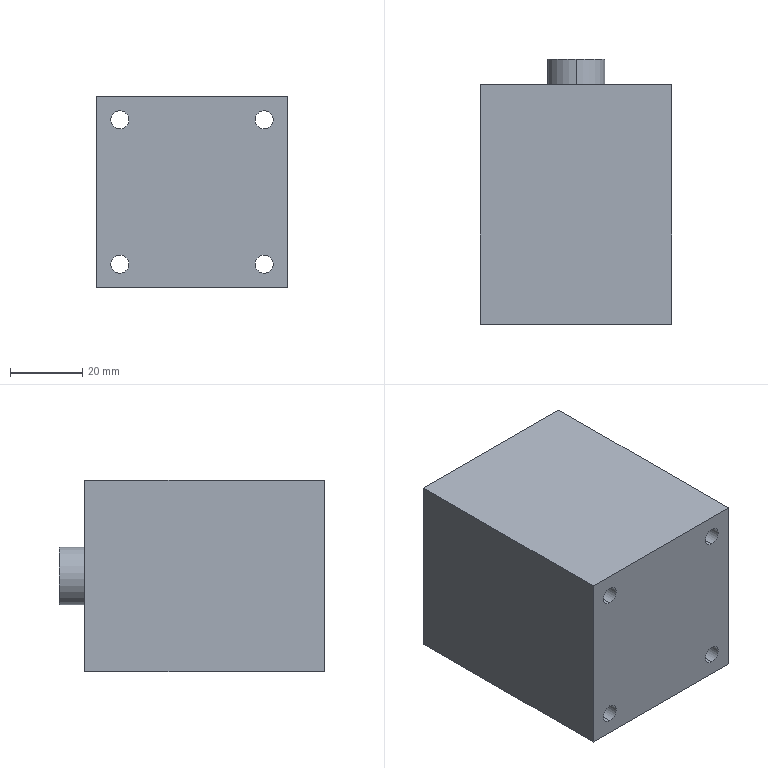Part | STEP file | 1 solid | 21 faces | box 53 x 73.5 x 53 mm | volume 182241 mm3 | cylinder 12 | plane 7 | cone 2 | commonest cylinder face diameters 5 x8 6.8 x2 16 x2
STEP:
#1=CARTESIAN_POINT('',(0.,0.,0.));
#2=DIRECTION('',(0.,0.,1.));
#3=DIRECTION('',(1.,0.,0.));
#4=AXIS2_PLACEMENT_3D('',#1,#2,#3);
#5=CARTESIAN_POINT('',(-20.,0.,-17.5));
#6=VERTEX_POINT('',#5);
#7=CARTESIAN_POINT('',(-20.,66.5,-17.5));
#8=VERTEX_POINT('',#7);
#9=CARTESIAN_POINT('',(-20.,66.5,-17.5));
#10=DIRECTION('',(0.,1.,0.));
#11=VECTOR('',#10,1.);
#12=LINE('',#9,#11);
#13=CARTESIAN_POINT('',(-20.,66.5,-20.));
#14=DIRECTION('',(0.,1.,0.));
#15=DIRECTION('',(0.,0.,1.));
#16=AXIS2_PLACEMENT_3D('',#13,#14,#15);
#17=CYLINDRICAL_SURFACE('',#16,2.5);
#18=CARTESIAN_POINT('',(6.283,0.));
#19=DIRECTION('',(0.,1.));
#20=VECTOR('',#19,1.);
#21=LINE('',#18,#20);
#22=(GEOMETRIC_REPRESENTATION_CONTEXT(2)PARAMETRIC_REPRESENTATION_CONTEXT()REPRESENTATION_CONTEXT('',''));
#23=DEFINITIONAL_REPRESENTATION('',(#21),#22);
#24=PCURVE('',#17,#23);
#25=CARTESIAN_POINT('',(-20.,66.5,-20.));
#26=DIRECTION('',(0.,1.,0.));
#27=DIRECTION('',(0.,0.,1.));
#28=AXIS2_PLACEMENT_3D('',#25,#26,#27);
#29=CYLINDRICAL_SURFACE('',#28,2.5);
#30=CARTESIAN_POINT('',(0.,0.));
#31=DIRECTION('',(0.,1.));
#32=VECTOR('',#31,1.);
#33=LINE('',#30,#32);
#34=(GEOMETRIC_REPRESENTATION_CONTEXT(2)PARAMETRIC_REPRESENTATION_CONTEXT()REPRESENTATION_CONTEXT('',''));
#35=DEFINITIONAL_REPRESENTATION('',(#33),#34);
#36=PCURVE('',#29,#35);
#37=SURFACE_CURVE('',#12,(#24,#36),.PCURVE_S1.);
#38=EDGE_CURVE('',#6,#8,#37,.T.);
#39=ORIENTED_EDGE('',*,*,#38,.T.);
#40=CARTESIAN_POINT('',(-20.,66.5,-22.5));
#41=VERTEX_POINT('',#40);
#42=CARTESIAN_POINT('',(-20.,66.5,-20.));
#43=DIRECTION('',(0.,1.,0.));
#44=DIRECTION('',(0.,0.,1.));
#45=AXIS2_PLACEMENT_3D('',#42,#43,#44);
#46=CIRCLE('',#45,2.5);
#47=CARTESIAN_POINT('',(0.,0.));
#48=DIRECTION('',(1.,0.));
#49=VECTOR('',#48,1.);
#50=LINE('',#47,#49);
#51=(GEOMETRIC_REPRESENTATION_CONTEXT(2)PARAMETRIC_REPRESENTATION_CONTEXT()REPRESENTATION_CONTEXT('',''));
#52=DEFINITIONAL_REPRESENTATION('',(#50),#51);
#53=PCURVE('',#17,#52);
#54=CARTESIAN_POINT('',(0.,66.5,0.));
#55=DIRECTION('',(0.,1.,0.));
#56=DIRECTION('',(0.,0.,1.));
#57=AXIS2_PLACEMENT_3D('',#54,#55,#56);
#58=PLANE('',#57);
#59=CARTESIAN_POINT('',(-20.,-20.));
#60=DIRECTION('',(1.,0.));
#61=AXIS2_PLACEMENT_2D('',#59,#60);
#62=CIRCLE('',#61,2.5);
#63=(GEOMETRIC_REPRESENTATION_CONTEXT(2)PARAMETRIC_REPRESENTATION_CONTEXT()REPRESENTATION_CONTEXT('',''));
#64=DEFINITIONAL_REPRESENTATION('',(#62),#63);
#65=PCURVE('',#58,#64);
#66=SURFACE_CURVE('',#46,(#53,#65),.PCURVE_S1.);
#67=EDGE_CURVE('',#41,#8,#66,.T.);
#68=ORIENTED_EDGE('',*,*,#67,.F.);
#69=CARTESIAN_POINT('',(-20.,0.,-22.5));
#70=VERTEX_POINT('',#69);
#71=CARTESIAN_POINT('',(-20.,66.5,-22.5));
#72=DIRECTION('',(0.,1.,0.));
#73=VECTOR('',#72,1.);
#74=LINE('',#71,#73);
#75=CARTESIAN_POINT('',(3.142,0.));
#76=DIRECTION('',(0.,1.));
#77=VECTOR('',#76,1.);
#78=LINE('',#75,#77);
#79=(GEOMETRIC_REPRESENTATION_CONTEXT(2)PARAMETRIC_REPRESENTATION_CONTEXT()REPRESENTATION_CONTEXT('',''));
#80=DEFINITIONAL_REPRESENTATION('',(#78),#79);
#81=PCURVE('',#17,#80);
#82=CARTESIAN_POINT('',(3.142,0.));
#83=DIRECTION('',(0.,1.));
#84=VECTOR('',#83,1.);
#85=LINE('',#82,#84);
#86=(GEOMETRIC_REPRESENTATION_CONTEXT(2)PARAMETRIC_REPRESENTATION_CONTEXT()REPRESENTATION_CONTEXT('',''));
#87=DEFINITIONAL_REPRESENTATION('',(#85),#86);
#88=PCURVE('',#29,#87);
#89=SURFACE_CURVE('',#74,(#81,#88),.PCURVE_S1.);
#90=EDGE_CURVE('',#70,#41,#89,.T.);
#91=ORIENTED_EDGE('',*,*,#90,.F.);
#92=CARTESIAN_POINT('',(-20.,0.,-20.));
#93=DIRECTION('',(0.,1.,0.));
#94=DIRECTION('',(0.,0.,1.));
#95=AXIS2_PLACEMENT_3D('',#92,#93,#94);
#96=CIRCLE('',#95,2.5);
#97=CARTESIAN_POINT('',(0.,-66.5));
#98=DIRECTION('',(1.,0.));
#99=VECTOR('',#98,1.);
#100=LINE('',#97,#99);
#101=(GEOMETRIC_REPRESENTATION_CONTEXT(2)PARAMETRIC_REPRESENTATION_CONTEXT()REPRESENTATION_CONTEXT('',''));
#102=DEFINITIONAL_REPRESENTATION('',(#100),#101);
#103=PCURVE('',#17,#102);
#104=CARTESIAN_POINT('',(0.,0.,0.));
#105=DIRECTION('',(0.,1.,0.));
#106=DIRECTION('',(0.,0.,1.));
#107=AXIS2_PLACEMENT_3D('',#104,#105,#106);
#108=PLANE('',#107);
#109=CARTESIAN_POINT('',(-20.,-20.));
#110=DIRECTION('',(1.,0.));
#111=AXIS2_PLACEMENT_2D('',#109,#110);
#112=CIRCLE('',#111,2.5);
#113=(GEOMETRIC_REPRESENTATION_CONTEXT(2)PARAMETRIC_REPRESENTATION_CONTEXT()REPRESENTATION_CONTEXT('',''));
#114=DEFINITIONAL_REPRESENTATION('',(#112),#113);
#115=PCURVE('',#108,#114);
#116=SURFACE_CURVE('',#96,(#103,#115),.PCURVE_S1.);
#117=EDGE_CURVE('',#70,#6,#116,.T.);
#118=ORIENTED_EDGE('',*,*,#117,.T.);
#119=EDGE_LOOP('',(#39,#68,#91,#118));
#120=FACE_BOUND('',#119,.F.);
#121=ADVANCED_FACE('',(#120),#17,.F.);
#122=CARTESIAN_POINT('',(-20.,0.,22.5));
#123=VERTEX_POINT('',#122);
#124=CARTESIAN_POINT('',(-20.,66.5,22.5));
#125=VERTEX_POINT('',#124);
#126=CARTESIAN_POINT('',(-20.,66.5,22.5));
#127=DIRECTION('',(0.,1.,0.));
#128=VECTOR('',#127,1.);
#129=LINE('',#126,#128);
#130=CARTESIAN_POINT('',(-20.,66.5,20.));
#131=DIRECTION('',(0.,1.,0.));
#132=DIRECTION('',(0.,0.,1.));
#133=AXIS2_PLACEMENT_3D('',#130,#131,#132);
#134=CYLINDRICAL_SURFACE('',#133,2.5);
#135=CARTESIAN_POINT('',(6.283,0.));
#136=DIRECTION('',(0.,1.));
#137=VECTOR('',#136,1.);
#138=LINE('',#135,#137);
#139=(GEOMETRIC_REPRESENTATION_CONTEXT(2)PARAMETRIC_REPRESENTATION_CONTEXT()REPRESENTATION_CONTEXT('',''));
#140=DEFINITIONAL_REPRESENTATION('',(#138),#139);
#141=PCURVE('',#134,#140);
#142=CARTESIAN_POINT('',(-20.,66.5,20.));
#143=DIRECTION('',(0.,1.,0.));
#144=DIRECTION('',(0.,0.,1.));
#145=AXIS2_PLACEMENT_3D('',#142,#143,#144);
#146=CYLINDRICAL_SURFACE('',#145,2.5);
#147=CARTESIAN_POINT('',(0.,0.));
#148=DIRECTION('',(0.,1.));
#149=VECTOR('',#148,1.);
#150=LINE('',#147,#149);
#151=(GEOMETRIC_REPRESENTATION_CONTEXT(2)PARAMETRIC_REPRESENTATION_CONTEXT()REPRESENTATION_CONTEXT('',''));
#152=DEFINITIONAL_REPRESENTATION('',(#150),#151);
#153=PCURVE('',#146,#152);
#154=SURFACE_CURVE('',#129,(#141,#153),.PCURVE_S1.);
#155=EDGE_CURVE('',#123,#125,#154,.T.);
#156=ORIENTED_EDGE('',*,*,#155,.T.);
#157=CARTESIAN_POINT('',(-20.,66.5,17.5));
#158=VERTEX_POINT('',#157);
#159=CARTESIAN_POINT('',(-20.,66.5,20.));
#160=DIRECTION('',(0.,1.,0.));
#161=DIRECTION('',(0.,0.,1.));
#162=AXIS2_PLACEMENT_3D('',#159,#160,#161);
#163=CIRCLE('',#162,2.5);
#164=CARTESIAN_POINT('',(0.,0.));
#165=DIRECTION('',(1.,0.));
#166=VECTOR('',#165,1.);
#167=LINE('',#164,#166);
#168=(GEOMETRIC_REPRESENTATION_CONTEXT(2)PARAMETRIC_REPRESENTATION_CONTEXT()REPRESENTATION_CONTEXT('',''));
#169=DEFINITIONAL_REPRESENTATION('',(#167),#168);
#170=PCURVE('',#134,#169);
#171=CARTESIAN_POINT('',(20.,-20.));
#172=DIRECTION('',(1.,0.));
#173=AXIS2_PLACEMENT_2D('',#171,#172);
#174=CIRCLE('',#173,2.5);
#175=(GEOMETRIC_REPRESENTATION_CONTEXT(2)PARAMETRIC_REPRESENTATION_CONTEXT()REPRESENTATION_CONTEXT('',''));
#176=DEFINITIONAL_REPRESENTATION('',(#174),#175);
#177=PCURVE('',#58,#176);
#178=SURFACE_CURVE('',#163,(#170,#177),.PCURVE_S1.);
#179=EDGE_CURVE('',#158,#125,#178,.T.);
#180=ORIENTED_EDGE('',*,*,#179,.F.);
#181=CARTESIAN_POINT('',(-20.,0.,17.5));
#182=VERTEX_POINT('',#181);
#183=CARTESIAN_POINT('',(-20.,66.5,17.5));
#184=DIRECTION('',(0.,1.,0.));
#185=VECTOR('',#184,1.);
#186=LINE('',#183,#185);
#187=CARTESIAN_POINT('',(3.142,0.));
#188=DIRECTION('',(0.,1.));
#189=VECTOR('',#188,1.);
#190=LINE('',#187,#189);
#191=(GEOMETRIC_REPRESENTATION_CONTEXT(2)PARAMETRIC_REPRESENTATION_CONTEXT()REPRESENTATION_CONTEXT('',''));
#192=DEFINITIONAL_REPRESENTATION('',(#190),#191);
#193=PCURVE('',#134,#192);
#194=CARTESIAN_POINT('',(3.142,0.));
#195=DIRECTION('',(0.,1.));
#196=VECTOR('',#195,1.);
#197=LINE('',#194,#196);
#198=(GEOMETRIC_REPRESENTATION_CONTEXT(2)PARAMETRIC_REPRESENTATION_CONTEXT()REPRESENTATION_CONTEXT('',''));
#199=DEFINITIONAL_REPRESENTATION('',(#197),#198);
#200=PCURVE('',#146,#199);
#201=SURFACE_CURVE('',#186,(#193,#200),.PCURVE_S1.);
#202=EDGE_CURVE('',#182,#158,#201,.T.);
#203=ORIENTED_EDGE('',*,*,#202,.F.);
#204=CARTESIAN_POINT('',(-20.,0.,20.));
#205=DIRECTION('',(0.,1.,0.));
#206=DIRECTION('',(0.,0.,1.));
#207=AXIS2_PLACEMENT_3D('',#204,#205,#206);
#208=CIRCLE('',#207,2.5);
#209=CARTESIAN_POINT('',(0.,-66.5));
#210=DIRECTION('',(1.,0.));
#211=VECTOR('',#210,1.);
#212=LINE('',#209,#211);
#213=(GEOMETRIC_REPRESENTATION_CONTEXT(2)PARAMETRIC_REPRESENTATION_CONTEXT()REPRESENTATION_CONTEXT('',''));
#214=DEFINITIONAL_REPRESENTATION('',(#212),#213);
#215=PCURVE('',#134,#214);
#216=CARTESIAN_POINT('',(20.,-20.));
#217=DIRECTION('',(1.,0.));
#218=AXIS2_PLACEMENT_2D('',#216,#217);
#219=CIRCLE('',#218,2.5);
#220=(GEOMETRIC_REPRESENTATION_CONTEXT(2)PARAMETRIC_REPRESENTATION_CONTEXT()REPRESENTATION_CONTEXT('',''));
#221=DEFINITIONAL_REPRESENTATION('',(#219),#220);
#222=PCURVE('',#108,#221);
#223=SURFACE_CURVE('',#208,(#215,#222),.PCURVE_S1.);
#224=EDGE_CURVE('',#182,#123,#223,.T.);
#225=ORIENTED_EDGE('',*,*,#224,.T.);
#226=EDGE_LOOP('',(#156,#180,#203,#225));
#227=FACE_BOUND('',#226,.F.);
#228=ADVANCED_FACE('',(#227),#134,.F.);
#229=CARTESIAN_POINT('',(20.,0.,22.5));
#230=VERTEX_POINT('',#229);
#231=CARTESIAN_POINT('',(20.,66.5,22.5));
#232=VERTEX_POINT('',#231);
#233=CARTESIAN_POINT('',(20.,66.5,22.5));
#234=DIRECTION('',(0.,1.,0.));
#235=VECTOR('',#234,1.);
#236=LINE('',#233,#235);
#237=CARTESIAN_POINT('',(20.,66.5,20.));
#238=DIRECTION('',(0.,1.,0.));
#239=DIRECTION('',(0.,0.,1.));
#240=AXIS2_PLACEMENT_3D('',#237,#238,#239);
#241=CYLINDRICAL_SURFACE('',#240,2.5);
#242=CARTESIAN_POINT('',(6.283,0.));
#243=DIRECTION('',(0.,1.));
#244=VECTOR('',#243,1.);
#245=LINE('',#242,#244);
#246=(GEOMETRIC_REPRESENTATION_CONTEXT(2)PARAMETRIC_REPRESENTATION_CONTEXT()REPRESENTATION_CONTEXT('',''));
#247=DEFINITIONAL_REPRESENTATION('',(#245),#246);
#248=PCURVE('',#241,#247);
#249=CARTESIAN_POINT('',(20.,66.5,20.));
#250=DIRECTION('',(0.,1.,0.));
#251=DIRECTION('',(0.,0.,1.));
#252=AXIS2_PLACEMENT_3D('',#249,#250,#251);
#253=CYLINDRICAL_SURFACE('',#252,2.5);
#254=CARTESIAN_POINT('',(0.,0.));
#255=DIRECTION('',(0.,1.));
#256=VECTOR('',#255,1.);
#257=LINE('',#254,#256);
#258=(GEOMETRIC_REPRESENTATION_CONTEXT(2)PARAMETRIC_REPRESENTATION_CONTEXT()REPRESENTATION_CONTEXT('',''));
#259=DEFINITIONAL_REPRESENTATION('',(#257),#258);
#260=PCURVE('',#253,#259);
#261=SURFACE_CURVE('',#236,(#248,#260),.PCURVE_S1.);
#262=EDGE_CURVE('',#230,#232,#261,.T.);
#263=ORIENTED_EDGE('',*,*,#262,.T.);
#264=CARTESIAN_POINT('',(20.,66.5,17.5));
#265=VERTEX_POINT('',#264);
#266=CARTESIAN_POINT('',(20.,66.5,20.));
#267=DIRECTION('',(0.,1.,0.));
#268=DIRECTION('',(0.,0.,1.));
#269=AXIS2_PLACEMENT_3D('',#266,#267,#268);
#270=CIRCLE('',#269,2.5);
#271=CARTESIAN_POINT('',(0.,0.));
#272=DIRECTION('',(1.,0.));
#273=VECTOR('',#272,1.);
#274=LINE('',#271,#273);
#275=(GEOMETRIC_REPRESENTATION_CONTEXT(2)PARAMETRIC_REPRESENTATION_CONTEXT()REPRESENTATION_CONTEXT('',''));
#276=DEFINITIONAL_REPRESENTATION('',(#274),#275);
#277=PCURVE('',#241,#276);
#278=CARTESIAN_POINT('',(20.,20.));
#279=DIRECTION('',(1.,0.));
#280=AXIS2_PLACEMENT_2D('',#278,#279);
#281=CIRCLE('',#280,2.5);
#282=(GEOMETRIC_REPRESENTATION_CONTEXT(2)PARAMETRIC_REPRESENTATION_CONTEXT()REPRESENTATION_CONTEXT('',''));
#283=DEFINITIONAL_REPRESENTATION('',(#281),#282);
#284=PCURVE('',#58,#283);
#285=SURFACE_CURVE('',#270,(#277,#284),.PCURVE_S1.);
#286=EDGE_CURVE('',#265,#232,#285,.T.);
#287=ORIENTED_EDGE('',*,*,#286,.F.);
#288=CARTESIAN_POINT('',(20.,0.,17.5));
#289=VERTEX_POINT('',#288);
#290=CARTESIAN_POINT('',(20.,66.5,17.5));
#291=DIRECTION('',(0.,1.,0.));
#292=VECTOR('',#291,1.);
#293=LINE('',#290,#292);
#294=CARTESIAN_POINT('',(3.142,0.));
#295=DIRECTION('',(0.,1.));
#296=VECTOR('',#295,1.);
#297=LINE('',#294,#296);
#298=(GEOMETRIC_REPRESENTATION_CONTEXT(2)PARAMETRIC_REPRESENTATION_CONTEXT()REPRESENTATION_CONTEXT('',''));
#299=DEFINITIONAL_REPRESENTATION('',(#297),#298);
#300=PCURVE('',#241,#299);
#301=CARTESIAN_POINT('',(3.142,0.));
#302=DIRECTION('',(0.,1.));
#303=VECTOR('',#302,1.);
#304=LINE('',#301,#303);
#305=(GEOMETRIC_REPRESENTATION_CONTEXT(2)PARAMETRIC_REPRESENTATION_CONTEXT()REPRESENTATION_CONTEXT('',''));
#306=DEFINITIONAL_REPRESENTATION('',(#304),#305);
#307=PCURVE('',#253,#306);
#308=SURFACE_CURVE('',#293,(#300,#307),.PCURVE_S1.);
#309=EDGE_CURVE('',#289,#265,#308,.T.);
#310=ORIENTED_EDGE('',*,*,#309,.F.);
#311=CARTESIAN_POINT('',(20.,0.,20.));
#312=DIRECTION('',(0.,1.,0.));
#313=DIRECTION('',(0.,0.,1.));
#314=AXIS2_PLACEMENT_3D('',#311,#312,#313);
#315=CIRCLE('',#314,2.5);
#316=CARTESIAN_POINT('',(0.,-66.5));
#317=DIRECTION('',(1.,0.));
#318=VECTOR('',#317,1.);
#319=LINE('',#316,#318);
#320=(GEOMETRIC_REPRESENTATION_CONTEXT(2)PARAMETRIC_REPRESENTATION_CONTEXT()REPRESENTATION_CONTEXT('',''));
#321=DEFINITIONAL_REPRESENTATION('',(#319),#320);
#322=PCURVE('',#241,#321);
#323=CARTESIAN_POINT('',(20.,20.));
#324=DIRECTION('',(1.,0.));
#325=AXIS2_PLACEMENT_2D('',#323,#324);
#326=CIRCLE('',#325,2.5);
#327=(GEOMETRIC_REPRESENTATION_CONTEXT(2)PARAMETRIC_REPRESENTATION_CONTEXT()REPRESENTATION_CONTEXT('',''));
#328=DEFINITIONAL_REPRESENTATION('',(#326),#327);
#329=PCURVE('',#108,#328);
#330=SURFACE_CURVE('',#315,(#322,#329),.PCURVE_S1.);
#331=EDGE_CURVE('',#289,#230,#330,.T.);
#332=ORIENTED_EDGE('',*,*,#331,.T.);
#333=EDGE_LOOP('',(#263,#287,#310,#332));
#334=FACE_BOUND('',#333,.F.);
#335=ADVANCED_FACE('',(#334),#241,.F.);
#336=CARTESIAN_POINT('',(20.,0.,-17.5));
#337=VERTEX_POINT('',#336);
#338=CARTESIAN_POINT('',(20.,66.5,-17.5));
#339=VERTEX_POINT('',#338);
#340=CARTESIAN_POINT('',(20.,66.5,-17.5));
#341=DIRECTION('',(0.,1.,0.));
#342=VECTOR('',#341,1.);
#343=LINE('',#340,#342);
#344=CARTESIAN_POINT('',(20.,66.5,-20.));
#345=DIRECTION('',(0.,1.,0.));
#346=DIRECTION('',(0.,0.,1.));
#347=AXIS2_PLACEMENT_3D('',#344,#345,#346);
#348=CYLINDRICAL_SURFACE('',#347,2.5);
#349=CARTESIAN_POINT('',(6.283,0.));
#350=DIRECTION('',(0.,1.));
#351=VECTOR('',#350,1.);
#352=LINE('',#349,#351);
#353=(GEOMETRIC_REPRESENTATION_CONTEXT(2)PARAMETRIC_REPRESENTATION_CONTEXT()REPRESENTATION_CONTEXT('',''));
#354=DEFINITIONAL_REPRESENTATION('',(#352),#353);
#355=PCURVE('',#348,#354);
#356=CARTESIAN_POINT('',(20.,66.5,-20.));
#357=DIRECTION('',(0.,1.,0.));
#358=DIRECTION('',(0.,0.,1.));
#359=AXIS2_PLACEMENT_3D('',#356,#357,#358);
#360=CYLINDRICAL_SURFACE('',#359,2.5);
#361=CARTESIAN_POINT('',(0.,0.));
#362=DIRECTION('',(0.,1.));
#363=VECTOR('',#362,1.);
#364=LINE('',#361,#363);
#365=(GEOMETRIC_REPRESENTATION_CONTEXT(2)PARAMETRIC_REPRESENTATION_CONTEXT()REPRESENTATION_CONTEXT('',''));
#366=DEFINITIONAL_REPRESENTATION('',(#364),#365);
#367=PCURVE('',#360,#366);
#368=SURFACE_CURVE('',#343,(#355,#367),.PCURVE_S1.);
#369=EDGE_CURVE('',#337,#339,#368,.T.);
#370=ORIENTED_EDGE('',*,*,#369,.T.);
#371=CARTESIAN_POINT('',(20.,66.5,-22.5));
#372=VERTEX_POINT('',#371);
#373=CARTESIAN_POINT('',(20.,66.5,-20.));
#374=DIRECTION('',(0.,1.,0.));
#375=DIRECTION('',(0.,0.,1.));
#376=AXIS2_PLACEMENT_3D('',#373,#374,#375);
#377=CIRCLE('',#376,2.5);
#378=CARTESIAN_POINT('',(0.,0.));
#379=DIRECTION('',(1.,0.));
#380=VECTOR('',#379,1.);
#381=LINE('',#378,#380);
#382=(GEOMETRIC_REPRESENTATION_CONTEXT(2)PARAMETRIC_REPRESENTATION_CONTEXT()REPRESENTATION_CONTEXT('',''));
#383=DEFINITIONAL_REPRESENTATION('',(#381),#382);
#384=PCURVE('',#348,#383);
#385=CARTESIAN_POINT('',(-20.,20.));
#386=DIRECTION('',(1.,0.));
#387=AXIS2_PLACEMENT_2D('',#385,#386);
#388=CIRCLE('',#387,2.5);
#389=(GEOMETRIC_REPRESENTATION_CONTEXT(2)PARAMETRIC_REPRESENTATION_CONTEXT()REPRESENTATION_CONTEXT('',''));
#390=DEFINITIONAL_REPRESENTATION('',(#388),#389);
#391=PCURVE('',#58,#390);
#392=SURFACE_CURVE('',#377,(#384,#391),.PCURVE_S1.);
#393=EDGE_CURVE('',#372,#339,#392,.T.);
#394=ORIENTED_EDGE('',*,*,#393,.F.);
#395=CARTESIAN_POINT('',(20.,0.,-22.5));
#396=VERTEX_POINT('',#395);
#397=CARTESIAN_POINT('',(20.,66.5,-22.5));
#398=DIRECTION('',(0.,1.,0.));
#399=VECTOR('',#398,1.);
#400=LINE('',#397,#399);
#401=CARTESIAN_POINT('',(3.142,0.));
#402=DIRECTION('',(0.,1.));
#403=VECTOR('',#402,1.);
#404=LINE('',#401,#403);
#405=(GEOMETRIC_REPRESENTATION_CONTEXT(2)PARAMETRIC_REPRESENTATION_CONTEXT()REPRESENTATION_CONTEXT('',''));
#406=DEFINITIONAL_REPRESENTATION('',(#404),#405);
#407=PCURVE('',#348,#406);
#408=CARTESIAN_POINT('',(3.142,0.));
#409=DIRECTION('',(0.,1.));
#410=VECTOR('',#409,1.);
#411=LINE('',#408,#410);
#412=(GEOMETRIC_REPRESENTATION_CONTEXT(2)PARAMETRIC_REPRESENTATION_CONTEXT()REPRESENTATION_CONTEXT('',''));
#413=DEFINITIONAL_REPRESENTATION('',(#411),#412);
#414=PCURVE('',#360,#413);
#415=SURFACE_CURVE('',#400,(#407,#414),.PCURVE_S1.);
#416=EDGE_CURVE('',#396,#372,#415,.T.);
#417=ORIENTED_EDGE('',*,*,#416,.F.);
#418=CARTESIAN_POINT('',(20.,0.,-20.));
#419=DIRECTION('',(0.,1.,0.));
#420=DIRECTION('',(0.,0.,1.));
#421=AXIS2_PLACEMENT_3D('',#418,#419,#420);
#422=CIRCLE('',#421,2.5);
#423=CARTESIAN_POINT('',(0.,-66.5));
#424=DIRECTION('',(1.,0.));
#425=VECTOR('',#424,1.);
#426=LINE('',#423,#425);
#427=(GEOMETRIC_REPRESENTATION_CONTEXT(2)PARAMETRIC_REPRESENTATION_CONTEXT()REPRESENTATION_CONTEXT('',''));
#428=DEFINITIONAL_REPRESENTATION('',(#426),#427);
#429=PCURVE('',#348,#428);
#430=CARTESIAN_POINT('',(-20.,20.));
#431=DIRECTION('',(1.,0.));
#432=AXIS2_PLACEMENT_2D('',#430,#431);
#433=CIRCLE('',#432,2.5);
#434=(GEOMETRIC_REPRESENTATION_CONTEXT(2)PARAMETRIC_REPRESENTATION_CONTEXT()REPRESENTATION_CONTEXT('',''));
#435=DEFINITIONAL_REPRESENTATION('',(#433),#434);
#436=PCURVE('',#108,#435);
#437=SURFACE_CURVE('',#422,(#429,#436),.PCURVE_S1.);
#438=EDGE_CURVE('',#396,#337,#437,.T.);
#439=ORIENTED_EDGE('',*,*,#438,.T.);
#440=EDGE_LOOP('',(#370,#394,#417,#439));
#441=FACE_BOUND('',#440,.F.);
#442=ADVANCED_FACE('',(#441),#348,.F.);
#443=CARTESIAN_POINT('',(0.,53.75,3.4));
#444=VERTEX_POINT('',#443);
#445=CARTESIAN_POINT('',(0.,73.5,3.4));
#446=VERTEX_POINT('',#445);
#447=CARTESIAN_POINT('',(0.,73.5,3.4));
#448=DIRECTION('',(0.,1.,0.));
#449=VECTOR('',#448,1.);
#450=LINE('',#447,#449);
#451=CARTESIAN_POINT('',(0.,73.5,0.));
#452=DIRECTION('',(0.,1.,0.));
#453=DIRECTION('',(0.,0.,1.));
#454=AXIS2_PLACEMENT_3D('',#451,#452,#453);
#455=CYLINDRICAL_SURFACE('',#454,3.4);
#456=CARTESIAN_POINT('',(6.283,0.));
#457=DIRECTION('',(0.,1.));
#458=VECTOR('',#457,1.);
#459=LINE('',#456,#458);
#460=(GEOMETRIC_REPRESENTATION_CONTEXT(2)PARAMETRIC_REPRESENTATION_CONTEXT()REPRESENTATION_CONTEXT('',''));
#461=DEFINITIONAL_REPRESENTATION('',(#459),#460);
#462=PCURVE('',#455,#461);
#463=CARTESIAN_POINT('',(0.,73.5,0.));
#464=DIRECTION('',(0.,1.,0.));
#465=DIRECTION('',(0.,0.,1.));
#466=AXIS2_PLACEMENT_3D('',#463,#464,#465);
#467=CYLINDRICAL_SURFACE('',#466,3.4);
#468=CARTESIAN_POINT('',(0.,0.));
#469=DIRECTION('',(0.,1.));
#470=VECTOR('',#469,1.);
#471=LINE('',#468,#470);
#472=(GEOMETRIC_REPRESENTATION_CONTEXT(2)PARAMETRIC_REPRESENTATION_CONTEXT()REPRESENTATION_CONTEXT('',''));
#473=DEFINITIONAL_REPRESENTATION('',(#471),#472);
#474=PCURVE('',#467,#473);
#475=SURFACE_CURVE('',#450,(#462,#474),.PCURVE_S1.);
#476=EDGE_CURVE('',#444,#446,#475,.T.);
#477=ORIENTED_EDGE('',*,*,#476,.T.);
#478=CARTESIAN_POINT('',(0.,73.5,-3.4));
#479=VERTEX_POINT('',#478);
#480=CARTESIAN_POINT('',(0.,73.5,0.));
#481=DIRECTION('',(0.,1.,0.));
#482=DIRECTION('',(0.,0.,1.));
#483=AXIS2_PLACEMENT_3D('',#480,#481,#482);
#484=CIRCLE('',#483,3.4);
#485=CARTESIAN_POINT('',(0.,0.));
#486=DIRECTION('',(1.,0.));
#487=VECTOR('',#486,1.);
#488=LINE('',#485,#487);
#489=(GEOMETRIC_REPRESENTATION_CONTEXT(2)PARAMETRIC_REPRESENTATION_CONTEXT()REPRESENTATION_CONTEXT('',''));
#490=DEFINITIONAL_REPRESENTATION('',(#488),#489);
#491=PCURVE('',#455,#490);
#492=CARTESIAN_POINT('',(0.,73.5,0.));
#493=DIRECTION('',(0.,1.,0.));
#494=DIRECTION('',(0.,0.,1.));
#495=AXIS2_PLACEMENT_3D('',#492,#493,#494);
#496=PLANE('',#495);
#497=CARTESIAN_POINT('',(0.,0.));
#498=DIRECTION('',(1.,0.));
#499=AXIS2_PLACEMENT_2D('',#497,#498);
#500=CIRCLE('',#499,3.4);
#501=(GEOMETRIC_REPRESENTATION_CONTEXT(2)PARAMETRIC_REPRESENTATION_CONTEXT()REPRESENTATION_CONTEXT('',''));
#502=DEFINITIONAL_REPRESENTATION('',(#500),#501);
#503=PCURVE('',#496,#502);
#504=SURFACE_CURVE('',#484,(#491,#503),.PCURVE_S1.);
#505=EDGE_CURVE('',#479,#446,#504,.T.);
#506=ORIENTED_EDGE('',*,*,#505,.F.);
#507=CARTESIAN_POINT('',(0.,53.75,-3.4));
#508=VERTEX_POINT('',#507);
#509=CARTESIAN_POINT('',(0.,73.5,-3.4));
#510=DIRECTION('',(0.,1.,0.));
#511=VECTOR('',#510,1.);
#512=LINE('',#509,#511);
#513=CARTESIAN_POINT('',(3.142,0.));
#514=DIRECTION('',(0.,1.));
#515=VECTOR('',#514,1.);
#516=LINE('',#513,#515);
#517=(GEOMETRIC_REPRESENTATION_CONTEXT(2)PARAMETRIC_REPRESENTATION_CONTEXT()REPRESENTATION_CONTEXT('',''));
#518=DEFINITIONAL_REPRESENTATION('',(#516),#517);
#519=PCURVE('',#455,#518);
#520=CARTESIAN_POINT('',(3.142,0.));
#521=DIRECTION('',(0.,1.));
#522=VECTOR('',#521,1.);
#523=LINE('',#520,#522);
#524=(GEOMETRIC_REPRESENTATION_CONTEXT(2)PARAMETRIC_REPRESENTATION_CONTEXT()REPRESENTATION_CONTEXT('',''));
#525=DEFINITIONAL_REPRESENTATION('',(#523),#524);
#526=PCURVE('',#467,#525);
#527=SURFACE_CURVE('',#512,(#519,#526),.PCURVE_S1.);
#528=EDGE_CURVE('',#508,#479,#527,.T.);
#529=ORIENTED_EDGE('',*,*,#528,.F.);
#530=CARTESIAN_POINT('',(0.,53.75,0.));
#531=DIRECTION('',(0.,1.,0.));
#532=DIRECTION('',(0.,0.,1.));
#533=AXIS2_PLACEMENT_3D('',#530,#531,#532);
#534=CIRCLE('',#533,3.4);
#535=CARTESIAN_POINT('',(0.,-19.75));
#536=DIRECTION('',(1.,0.));
#537=VECTOR('',#536,1.);
#538=LINE('',#535,#537);
#539=(GEOMETRIC_REPRESENTATION_CONTEXT(2)PARAMETRIC_REPRESENTATION_CONTEXT()REPRESENTATION_CONTEXT('',''));
#540=DEFINITIONAL_REPRESENTATION('',(#538),#539);
#541=PCURVE('',#455,#540);
#542=CARTESIAN_POINT('',(0.,53.75,0.));
#543=DIRECTION('',(0.,1.,0.));
#544=DIRECTION('',(0.,0.,1.));
#545=AXIS2_PLACEMENT_3D('',#542,#543,#544);
#546=CONICAL_SURFACE('',#545,3.4,1.03);
#547=CARTESIAN_POINT('',(0.,0.));
#548=DIRECTION('',(1.,0.));
#549=VECTOR('',#548,1.);
#550=LINE('',#547,#549);
#551=(GEOMETRIC_REPRESENTATION_CONTEXT(2)PARAMETRIC_REPRESENTATION_CONTEXT()REPRESENTATION_CONTEXT('',''));
#552=DEFINITIONAL_REPRESENTATION('',(#550),#551);
#553=PCURVE('',#546,#552);
#554=SURFACE_CURVE('',#534,(#541,#553),.PCURVE_S1.);
#555=EDGE_CURVE('',#508,#444,#554,.T.);
#556=ORIENTED_EDGE('',*,*,#555,.T.);
#557=EDGE_LOOP('',(#477,#506,#529,#556));
#558=FACE_BOUND('',#557,.F.);
#559=ADVANCED_FACE('',(#558),#455,.F.);
#560=ORIENTED_EDGE('',*,*,#555,.F.);
#561=CARTESIAN_POINT('',(0.,51.707,0.));
#562=VERTEX_POINT('',#561);
#563=CARTESIAN_POINT('',(0.,53.75,-3.4));
#564=DIRECTION('',(0.,0.515,-0.8572));
#565=VECTOR('',#564,1.);
#566=LINE('',#563,#565);
#567=CARTESIAN_POINT('',(3.142,0.));
#568=DIRECTION('',(0.,1.));
#569=VECTOR('',#568,1.);
#570=LINE('',#567,#569);
#571=(GEOMETRIC_REPRESENTATION_CONTEXT(2)PARAMETRIC_REPRESENTATION_CONTEXT()REPRESENTATION_CONTEXT('',''));
#572=DEFINITIONAL_REPRESENTATION('',(#570),#571);
#573=PCURVE('',#546,#572);
#574=CARTESIAN_POINT('',(0.,53.75,0.));
#575=DIRECTION('',(0.,1.,0.));
#576=DIRECTION('',(0.,0.,1.));
#577=AXIS2_PLACEMENT_3D('',#574,#575,#576);
#578=CONICAL_SURFACE('',#577,3.4,1.03);
#579=CARTESIAN_POINT('',(3.142,0.));
#580=DIRECTION('',(0.,1.));
#581=VECTOR('',#580,1.);
#582=LINE('',#579,#581);
#583=(GEOMETRIC_REPRESENTATION_CONTEXT(2)PARAMETRIC_REPRESENTATION_CONTEXT()REPRESENTATION_CONTEXT('',''));
#584=DEFINITIONAL_REPRESENTATION('',(#582),#583);
#585=PCURVE('',#578,#584);
#586=SURFACE_CURVE('',#566,(#573,#585),.PCURVE_S1.);
#587=EDGE_CURVE('',#562,#508,#586,.T.);
#588=ORIENTED_EDGE('',*,*,#587,.F.);
#589=CARTESIAN_POINT('',(0.,53.75,3.4));
#590=DIRECTION('',(0.,0.515,0.8572));
#591=VECTOR('',#590,1.);
#592=LINE('',#589,#591);
#593=CARTESIAN_POINT('',(6.283,0.));
#594=DIRECTION('',(0.,1.));
#595=VECTOR('',#594,1.);
#596=LINE('',#593,#595);
#597=(GEOMETRIC_REPRESENTATION_CONTEXT(2)PARAMETRIC_REPRESENTATION_CONTEXT()REPRESENTATION_CONTEXT('',''));
#598=DEFINITIONAL_REPRESENTATION('',(#596),#597);
#599=PCURVE('',#546,#598);
#600=CARTESIAN_POINT('',(0.,0.));
#601=DIRECTION('',(0.,1.));
#602=VECTOR('',#601,1.);
#603=LINE('',#600,#602);
#604=(GEOMETRIC_REPRESENTATION_CONTEXT(2)PARAMETRIC_REPRESENTATION_CONTEXT()REPRESENTATION_CONTEXT('',''));
#605=DEFINITIONAL_REPRESENTATION('',(#603),#604);
#606=PCURVE('',#578,#605);
#607=SURFACE_CURVE('',#592,(#599,#606),.PCURVE_S1.);
#608=EDGE_CURVE('',#562,#444,#607,.T.);
#609=ORIENTED_EDGE('',*,*,#608,.T.);
#610=EDGE_LOOP('',(#560,#588,#609));
#611=FACE_BOUND('',#610,.F.);
#612=ADVANCED_FACE('',(#611),#546,.F.);
#613=CARTESIAN_POINT('',(0.,73.5,8.));
#614=VERTEX_POINT('',#613);
#615=CARTESIAN_POINT('',(0.,73.5,-8.));
#616=VERTEX_POINT('',#615);
#617=CARTESIAN_POINT('',(0.,73.5,0.));
#618=DIRECTION('',(0.,1.,0.));
#619=DIRECTION('',(0.,0.,1.));
#620=AXIS2_PLACEMENT_3D('',#617,#618,#619);
#621=CIRCLE('',#620,8.);
#622=CARTESIAN_POINT('',(0.,73.5,0.));
#623=DIRECTION('',(0.,-1.,0.));
#624=DIRECTION('',(0.,0.,-1.));
#625=AXIS2_PLACEMENT_3D('',#622,#623,#624);
#626=CYLINDRICAL_SURFACE('',#625,8.);
#627=CARTESIAN_POINT('',(3.142,0.));
#628=DIRECTION('',(-1.,0.));
#629=VECTOR('',#628,1.);
#630=LINE('',#627,#629);
#631=(GEOMETRIC_REPRESENTATION_CONTEXT(2)PARAMETRIC_REPRESENTATION_CONTEXT()REPRESENTATION_CONTEXT('',''));
#632=DEFINITIONAL_REPRESENTATION('',(#630),#631);
#633=PCURVE('',#626,#632);
#634=CARTESIAN_POINT('',(0.,0.));
#635=DIRECTION('',(1.,0.));
#636=AXIS2_PLACEMENT_2D('',#634,#635);
#637=CIRCLE('',#636,8.);
#638=(GEOMETRIC_REPRESENTATION_CONTEXT(2)PARAMETRIC_REPRESENTATION_CONTEXT()REPRESENTATION_CONTEXT('',''));
#639=DEFINITIONAL_REPRESENTATION('',(#637),#638);
#640=PCURVE('',#496,#639);
#641=SURFACE_CURVE('',#621,(#633,#640),.PCURVE_S1.);
#642=EDGE_CURVE('',#614,#616,#641,.T.);
#643=ORIENTED_EDGE('',*,*,#642,.F.);
#644=CARTESIAN_POINT('',(0.,66.5,8.));
#645=VERTEX_POINT('',#644);
#646=CARTESIAN_POINT('',(0.,73.5,8.));
#647=DIRECTION('',(0.,-1.,0.));
#648=VECTOR('',#647,1.);
#649=LINE('',#646,#648);
#650=CARTESIAN_POINT('',(3.142,0.));
#651=DIRECTION('',(0.,1.));
#652=VECTOR('',#651,1.);
#653=LINE('',#650,#652);
#654=(GEOMETRIC_REPRESENTATION_CONTEXT(2)PARAMETRIC_REPRESENTATION_CONTEXT()REPRESENTATION_CONTEXT('',''));
#655=DEFINITIONAL_REPRESENTATION('',(#653),#654);
#656=PCURVE('',#626,#655);
#657=CARTESIAN_POINT('',(0.,73.5,0.));
#658=DIRECTION('',(0.,-1.,0.));
#659=DIRECTION('',(0.,0.,-1.));
#660=AXIS2_PLACEMENT_3D('',#657,#658,#659);
#661=CYLINDRICAL_SURFACE('',#660,8.);
#662=CARTESIAN_POINT('',(3.142,0.));
#663=DIRECTION('',(0.,1.));
#664=VECTOR('',#663,1.);
#665=LINE('',#662,#664);
#666=(GEOMETRIC_REPRESENTATION_CONTEXT(2)PARAMETRIC_REPRESENTATION_CONTEXT()REPRESENTATION_CONTEXT('',''));
#667=DEFINITIONAL_REPRESENTATION('',(#665),#666);
#668=PCURVE('',#661,#667);
#669=SURFACE_CURVE('',#649,(#656,#668),.PCURVE_S1.);
#670=EDGE_CURVE('',#614,#645,#669,.T.);
#671=ORIENTED_EDGE('',*,*,#670,.T.);
#672=CARTESIAN_POINT('',(0.,66.5,-8.));
#673=VERTEX_POINT('',#672);
#674=CARTESIAN_POINT('',(0.,66.5,0.));
#675=DIRECTION('',(0.,1.,0.));
#676=DIRECTION('',(0.,0.,1.));
#677=AXIS2_PLACEMENT_3D('',#674,#675,#676);
#678=CIRCLE('',#677,8.);
#679=CARTESIAN_POINT('',(3.142,7.));
#680=DIRECTION('',(-1.,0.));
#681=VECTOR('',#680,1.);
#682=LINE('',#679,#681);
#683=(GEOMETRIC_REPRESENTATION_CONTEXT(2)PARAMETRIC_REPRESENTATION_CONTEXT()REPRESENTATION_CONTEXT('',''));
#684=DEFINITIONAL_REPRESENTATION('',(#682),#683);
#685=PCURVE('',#626,#684);
#686=CARTESIAN_POINT('',(0.,0.));
#687=DIRECTION('',(1.,0.));
#688=AXIS2_PLACEMENT_2D('',#686,#687);
#689=CIRCLE('',#688,8.);
#690=(GEOMETRIC_REPRESENTATION_CONTEXT(2)PARAMETRIC_REPRESENTATION_CONTEXT()REPRESENTATION_CONTEXT('',''));
#691=DEFINITIONAL_REPRESENTATION('',(#689),#690);
#692=PCURVE('',#58,#691);
#693=SURFACE_CURVE('',#678,(#685,#692),.PCURVE_S1.);
#694=EDGE_CURVE('',#645,#673,#693,.T.);
#695=ORIENTED_EDGE('',*,*,#694,.T.);
#696=CARTESIAN_POINT('',(0.,73.5,-8.));
#697=DIRECTION('',(0.,-1.,0.));
#698=VECTOR('',#697,1.);
#699=LINE('',#696,#698);
#700=CARTESIAN_POINT('',(0.,0.));
#701=DIRECTION('',(0.,1.));
#702=VECTOR('',#701,1.);
#703=LINE('',#700,#702);
#704=(GEOMETRIC_REPRESENTATION_CONTEXT(2)PARAMETRIC_REPRESENTATION_CONTEXT()REPRESENTATION_CONTEXT('',''));
#705=DEFINITIONAL_REPRESENTATION('',(#703),#704);
#706=PCURVE('',#626,#705);
#707=CARTESIAN_POINT('',(6.283,0.));
#708=DIRECTION('',(0.,1.));
#709=VECTOR('',#708,1.);
#710=LINE('',#707,#709);
#711=(GEOMETRIC_REPRESENTATION_CONTEXT(2)PARAMETRIC_REPRESENTATION_CONTEXT()REPRESENTATION_CONTEXT('',''));
#712=DEFINITIONAL_REPRESENTATION('',(#710),#711);
#713=PCURVE('',#661,#712);
#714=SURFACE_CURVE('',#699,(#706,#713),.PCURVE_S1.);
#715=EDGE_CURVE('',#616,#673,#714,.T.);
#716=ORIENTED_EDGE('',*,*,#715,.F.);
#717=EDGE_LOOP('',(#643,#671,#695,#716));
#718=FACE_BOUND('',#717,.T.);
#719=ADVANCED_FACE('',(#718),#626,.T.);
#720=CARTESIAN_POINT('',(-20.,66.5,-20.));
#721=DIRECTION('',(0.,1.,0.));
#722=DIRECTION('',(0.,0.,1.));
#723=AXIS2_PLACEMENT_3D('',#720,#721,#722);
#724=CIRCLE('',#723,2.5);
#725=CARTESIAN_POINT('',(-20.,-20.));
#726=DIRECTION('',(1.,0.));
#727=AXIS2_PLACEMENT_2D('',#725,#726);
#728=CIRCLE('',#727,2.5);
#729=(GEOMETRIC_REPRESENTATION_CONTEXT(2)PARAMETRIC_REPRESENTATION_CONTEXT()REPRESENTATION_CONTEXT('',''));
#730=DEFINITIONAL_REPRESENTATION('',(#728),#729);
#731=PCURVE('',#58,#730);
#732=CARTESIAN_POINT('',(0.,0.));
#733=DIRECTION('',(1.,0.));
#734=VECTOR('',#733,1.);
#735=LINE('',#732,#734);
#736=(GEOMETRIC_REPRESENTATION_CONTEXT(2)PARAMETRIC_REPRESENTATION_CONTEXT()REPRESENTATION_CONTEXT('',''));
#737=DEFINITIONAL_REPRESENTATION('',(#735),#736);
#738=PCURVE('',#29,#737);
#739=SURFACE_CURVE('',#724,(#731,#738),.PCURVE_S1.);
#740=EDGE_CURVE('',#8,#41,#739,.T.);
#741=ORIENTED_EDGE('',*,*,#740,.F.);
#742=ORIENTED_EDGE('',*,*,#67,.F.);
#743=EDGE_LOOP('',(#741,#742));
#744=FACE_BOUND('',#743,.T.);
#745=CARTESIAN_POINT('',(-20.,66.5,20.));
#746=DIRECTION('',(0.,1.,0.));
#747=DIRECTION('',(0.,0.,1.));
#748=AXIS2_PLACEMENT_3D('',#745,#746,#747);
#749=CIRCLE('',#748,2.5);
#750=CARTESIAN_POINT('',(20.,-20.));
#751=DIRECTION('',(1.,0.));
#752=AXIS2_PLACEMENT_2D('',#750,#751);
#753=CIRCLE('',#752,2.5);
#754=(GEOMETRIC_REPRESENTATION_CONTEXT(2)PARAMETRIC_REPRESENTATION_CONTEXT()REPRESENTATION_CONTEXT('',''));
#755=DEFINITIONAL_REPRESENTATION('',(#753),#754);
#756=PCURVE('',#58,#755);
#757=CARTESIAN_POINT('',(0.,0.));
#758=DIRECTION('',(1.,0.));
#759=VECTOR('',#758,1.);
#760=LINE('',#757,#759);
#761=(GEOMETRIC_REPRESENTATION_CONTEXT(2)PARAMETRIC_REPRESENTATION_CONTEXT()REPRESENTATION_CONTEXT('',''));
#762=DEFINITIONAL_REPRESENTATION('',(#760),#761);
#763=PCURVE('',#146,#762);
#764=SURFACE_CURVE('',#749,(#756,#763),.PCURVE_S1.);
#765=EDGE_CURVE('',#125,#158,#764,.T.);
#766=ORIENTED_EDGE('',*,*,#765,.F.);
#767=ORIENTED_EDGE('',*,*,#179,.F.);
#768=EDGE_LOOP('',(#766,#767));
#769=FACE_BOUND('',#768,.T.);
#770=CARTESIAN_POINT('',(20.,66.5,20.));
#771=DIRECTION('',(0.,1.,0.));
#772=DIRECTION('',(0.,0.,1.));
#773=AXIS2_PLACEMENT_3D('',#770,#771,#772);
#774=CIRCLE('',#773,2.5);
#775=CARTESIAN_POINT('',(20.,20.));
#776=DIRECTION('',(1.,0.));
#777=AXIS2_PLACEMENT_2D('',#775,#776);
#778=CIRCLE('',#777,2.5);
#779=(GEOMETRIC_REPRESENTATION_CONTEXT(2)PARAMETRIC_REPRESENTATION_CONTEXT()REPRESENTATION_CONTEXT('',''));
#780=DEFINITIONAL_REPRESENTATION('',(#778),#779);
#781=PCURVE('',#58,#780);
#782=CARTESIAN_POINT('',(0.,0.));
#783=DIRECTION('',(1.,0.));
#784=VECTOR('',#783,1.);
#785=LINE('',#782,#784);
#786=(GEOMETRIC_REPRESENTATION_CONTEXT(2)PARAMETRIC_REPRESENTATION_CONTEXT()REPRESENTATION_CONTEXT('',''));
#787=DEFINITIONAL_REPRESENTATION('',(#785),#786);
#788=PCURVE('',#253,#787);
#789=SURFACE_CURVE('',#774,(#781,#788),.PCURVE_S1.);
#790=EDGE_CURVE('',#232,#265,#789,.T.);
#791=ORIENTED_EDGE('',*,*,#790,.F.);
#792=ORIENTED_EDGE('',*,*,#286,.F.);
#793=EDGE_LOOP('',(#791,#792));
#794=FACE_BOUND('',#793,.T.);
#795=CARTESIAN_POINT('',(20.,66.5,-20.));
#796=DIRECTION('',(0.,1.,0.));
#797=DIRECTION('',(0.,0.,1.));
#798=AXIS2_PLACEMENT_3D('',#795,#796,#797);
#799=CIRCLE('',#798,2.5);
#800=CARTESIAN_POINT('',(-20.,20.));
#801=DIRECTION('',(1.,0.));
#802=AXIS2_PLACEMENT_2D('',#800,#801);
#803=CIRCLE('',#802,2.5);
#804=(GEOMETRIC_REPRESENTATION_CONTEXT(2)PARAMETRIC_REPRESENTATION_CONTEXT()REPRESENTATION_CONTEXT('',''));
#805=DEFINITIONAL_REPRESENTATION('',(#803),#804);
#806=PCURVE('',#58,#805);
#807=CARTESIAN_POINT('',(0.,0.));
#808=DIRECTION('',(1.,0.));
#809=VECTOR('',#808,1.);
#810=LINE('',#807,#809);
#811=(GEOMETRIC_REPRESENTATION_CONTEXT(2)PARAMETRIC_REPRESENTATION_CONTEXT()REPRESENTATION_CONTEXT('',''));
#812=DEFINITIONAL_REPRESENTATION('',(#810),#811);
#813=PCURVE('',#360,#812);
#814=SURFACE_CURVE('',#799,(#806,#813),.PCURVE_S1.);
#815=EDGE_CURVE('',#339,#372,#814,.T.);
#816=ORIENTED_EDGE('',*,*,#815,.F.);
#817=ORIENTED_EDGE('',*,*,#393,.F.);
#818=EDGE_LOOP('',(#816,#817));
#819=FACE_BOUND('',#818,.T.);
#820=CARTESIAN_POINT('',(-26.5,66.5,-26.5));
#821=VERTEX_POINT('',#820);
#822=CARTESIAN_POINT('',(-26.5,66.5,26.5));
#823=VERTEX_POINT('',#822);
#824=CARTESIAN_POINT('',(-26.5,66.5,26.5));
#825=DIRECTION('',(0.,0.,1.));
#826=VECTOR('',#825,1.);
#827=LINE('',#824,#826);
#828=CARTESIAN_POINT('',(26.5,-26.5));
#829=DIRECTION('',(1.,0.));
#830=VECTOR('',#829,1.);
#831=LINE('',#828,#830);
#832=(GEOMETRIC_REPRESENTATION_CONTEXT(2)PARAMETRIC_REPRESENTATION_CONTEXT()REPRESENTATION_CONTEXT('',''));
#833=DEFINITIONAL_REPRESENTATION('',(#831),#832);
#834=PCURVE('',#58,#833);
#835=CARTESIAN_POINT('',(-26.5,66.5,26.5));
#836=DIRECTION('',(1.,0.,0.));
#837=DIRECTION('',(0.,0.,-1.));
#838=AXIS2_PLACEMENT_3D('',#835,#836,#837);
#839=PLANE('',#838);
#840=CARTESIAN_POINT('',(0.,0.));
#841=DIRECTION('',(-1.,0.));
#842=VECTOR('',#841,1.);
#843=LINE('',#840,#842);
#844=(GEOMETRIC_REPRESENTATION_CONTEXT(2)PARAMETRIC_REPRESENTATION_CONTEXT()REPRESENTATION_CONTEXT('',''));
#845=DEFINITIONAL_REPRESENTATION('',(#843),#844);
#846=PCURVE('',#839,#845);
#847=SURFACE_CURVE('',#827,(#834,#846),.PCURVE_S1.);
#848=EDGE_CURVE('',#821,#823,#847,.T.);
#849=ORIENTED_EDGE('',*,*,#848,.T.);
#850=CARTESIAN_POINT('',(26.5,66.5,26.5));
#851=VERTEX_POINT('',#850);
#852=CARTESIAN_POINT('',(26.5,66.5,26.5));
#853=DIRECTION('',(1.,0.,0.));
#854=VECTOR('',#853,1.);
#855=LINE('',#852,#854);
#856=CARTESIAN_POINT('',(26.5,26.5));
#857=DIRECTION('',(0.,1.));
#858=VECTOR('',#857,1.);
#859=LINE('',#856,#858);
#860=(GEOMETRIC_REPRESENTATION_CONTEXT(2)PARAMETRIC_REPRESENTATION_CONTEXT()REPRESENTATION_CONTEXT('',''));
#861=DEFINITIONAL_REPRESENTATION('',(#859),#860);
#862=PCURVE('',#58,#861);
#863=CARTESIAN_POINT('',(26.5,66.5,26.5));
#864=DIRECTION('',(0.,0.,-1.));
#865=DIRECTION('',(-1.,0.,0.));
#866=AXIS2_PLACEMENT_3D('',#863,#864,#865);
#867=PLANE('',#866);
#868=CARTESIAN_POINT('',(0.,0.));
#869=DIRECTION('',(-1.,0.));
#870=VECTOR('',#869,1.);
#871=LINE('',#868,#870);
#872=(GEOMETRIC_REPRESENTATION_CONTEXT(2)PARAMETRIC_REPRESENTATION_CONTEXT()REPRESENTATION_CONTEXT('',''));
#873=DEFINITIONAL_REPRESENTATION('',(#871),#872);
#874=PCURVE('',#867,#873);
#875=SURFACE_CURVE('',#855,(#862,#874),.PCURVE_S1.);
#876=EDGE_CURVE('',#823,#851,#875,.T.);
#877=ORIENTED_EDGE('',*,*,#876,.T.);
#878=CARTESIAN_POINT('',(26.5,66.5,-26.5));
#879=VERTEX_POINT('',#878);
#880=CARTESIAN_POINT('',(26.5,66.5,26.5));
#881=DIRECTION('',(0.,0.,-1.));
#882=VECTOR('',#881,1.);
#883=LINE('',#880,#882);
#884=CARTESIAN_POINT('',(26.5,26.5));
#885=DIRECTION('',(-1.,0.));
#886=VECTOR('',#885,1.);
#887=LINE('',#884,#886);
#888=(GEOMETRIC_REPRESENTATION_CONTEXT(2)PARAMETRIC_REPRESENTATION_CONTEXT()REPRESENTATION_CONTEXT('',''));
#889=DEFINITIONAL_REPRESENTATION('',(#887),#888);
#890=PCURVE('',#58,#889);
#891=CARTESIAN_POINT('',(26.5,66.5,26.5));
#892=DIRECTION('',(-1.,0.,0.));
#893=DIRECTION('',(0.,0.,1.));
#894=AXIS2_PLACEMENT_3D('',#891,#892,#893);
#895=PLANE('',#894);
#896=CARTESIAN_POINT('',(0.,0.));
#897=DIRECTION('',(-1.,0.));
#898=VECTOR('',#897,1.);
#899=LINE('',#896,#898);
#900=(GEOMETRIC_REPRESENTATION_CONTEXT(2)PARAMETRIC_REPRESENTATION_CONTEXT()REPRESENTATION_CONTEXT('',''));
#901=DEFINITIONAL_REPRESENTATION('',(#899),#900);
#902=PCURVE('',#895,#901);
#903=SURFACE_CURVE('',#883,(#890,#902),.PCURVE_S1.);
#904=EDGE_CURVE('',#851,#879,#903,.T.);
#905=ORIENTED_EDGE('',*,*,#904,.T.);
#906=CARTESIAN_POINT('',(26.5,66.5,-26.5));
#907=DIRECTION('',(-1.,0.,0.));
#908=VECTOR('',#907,1.);
#909=LINE('',#906,#908);
#910=CARTESIAN_POINT('',(-26.5,26.5));
#911=DIRECTION('',(0.,-1.));
#912=VECTOR('',#911,1.);
#913=LINE('',#910,#912);
#914=(GEOMETRIC_REPRESENTATION_CONTEXT(2)PARAMETRIC_REPRESENTATION_CONTEXT()REPRESENTATION_CONTEXT('',''));
#915=DEFINITIONAL_REPRESENTATION('',(#913),#914);
#916=PCURVE('',#58,#915);
#917=CARTESIAN_POINT('',(26.5,66.5,-26.5));
#918=DIRECTION('',(0.,0.,1.));
#919=DIRECTION('',(1.,0.,0.));
#920=AXIS2_PLACEMENT_3D('',#917,#918,#919);
#921=PLANE('',#920);
#922=CARTESIAN_POINT('',(0.,0.));
#923=DIRECTION('',(-1.,0.));
#924=VECTOR('',#923,1.);
#925=LINE('',#922,#924);
#926=(GEOMETRIC_REPRESENTATION_CONTEXT(2)PARAMETRIC_REPRESENTATION_CONTEXT()REPRESENTATION_CONTEXT('',''));
#927=DEFINITIONAL_REPRESENTATION('',(#925),#926);
#928=PCURVE('',#921,#927);
#929=SURFACE_CURVE('',#909,(#916,#928),.PCURVE_S1.);
#930=EDGE_CURVE('',#879,#821,#929,.T.);
#931=ORIENTED_EDGE('',*,*,#930,.T.);
#932=EDGE_LOOP('',(#849,#877,#905,#931));
#933=FACE_BOUND('',#932,.T.);
#934=CARTESIAN_POINT('',(0.,66.5,0.));
#935=DIRECTION('',(0.,1.,0.));
#936=DIRECTION('',(0.,0.,1.));
#937=AXIS2_PLACEMENT_3D('',#934,#935,#936);
#938=CIRCLE('',#937,8.);
#939=CARTESIAN_POINT('',(0.,0.));
#940=DIRECTION('',(1.,0.));
#941=AXIS2_PLACEMENT_2D('',#939,#940);
#942=CIRCLE('',#941,8.);
#943=(GEOMETRIC_REPRESENTATION_CONTEXT(2)PARAMETRIC_REPRESENTATION_CONTEXT()REPRESENTATION_CONTEXT('',''));
#944=DEFINITIONAL_REPRESENTATION('',(#942),#943);
#945=PCURVE('',#58,#944);
#946=CARTESIAN_POINT('',(9.425,7.));
#947=DIRECTION('',(-1.,0.));
#948=VECTOR('',#947,1.);
#949=LINE('',#946,#948);
#950=(GEOMETRIC_REPRESENTATION_CONTEXT(2)PARAMETRIC_REPRESENTATION_CONTEXT()REPRESENTATION_CONTEXT('',''));
#951=DEFINITIONAL_REPRESENTATION('',(#949),#950);
#952=PCURVE('',#661,#951);
#953=SURFACE_CURVE('',#938,(#945,#952),.PCURVE_S1.);
#954=EDGE_CURVE('',#673,#645,#953,.T.);
#955=ORIENTED_EDGE('',*,*,#954,.F.);
#956=ORIENTED_EDGE('',*,*,#694,.F.);
#957=EDGE_LOOP('',(#955,#956));
#958=FACE_BOUND('',#957,.T.);
#959=ADVANCED_FACE('',(#744,#769,#794,#819,#933,#958),#58,.T.);
#960=CARTESIAN_POINT('',(-26.5,0.,-26.5));
#961=VERTEX_POINT('',#960);
#962=CARTESIAN_POINT('',(-26.5,0.,26.5));
#963=VERTEX_POINT('',#962);
#964=CARTESIAN_POINT('',(-26.5,0.,26.5));
#965=DIRECTION('',(0.,0.,1.));
#966=VECTOR('',#965,1.);
#967=LINE('',#964,#966);
#968=CARTESIAN_POINT('',(0.,-66.5));
#969=DIRECTION('',(-1.,0.));
#970=VECTOR('',#969,1.);
#971=LINE('',#968,#970);
#972=(GEOMETRIC_REPRESENTATION_CONTEXT(2)PARAMETRIC_REPRESENTATION_CONTEXT()REPRESENTATION_CONTEXT('',''));
#973=DEFINITIONAL_REPRESENTATION('',(#971),#972);
#974=PCURVE('',#839,#973);
#975=CARTESIAN_POINT('',(26.5,-26.5));
#976=DIRECTION('',(1.,0.));
#977=VECTOR('',#976,1.);
#978=LINE('',#975,#977);
#979=(GEOMETRIC_REPRESENTATION_CONTEXT(2)PARAMETRIC_REPRESENTATION_CONTEXT()REPRESENTATION_CONTEXT('',''));
#980=DEFINITIONAL_REPRESENTATION('',(#978),#979);
#981=PCURVE('',#108,#980);
#982=SURFACE_CURVE('',#967,(#974,#981),.PCURVE_S1.);
#983=EDGE_CURVE('',#961,#963,#982,.T.);
#984=ORIENTED_EDGE('',*,*,#983,.T.);
#985=CARTESIAN_POINT('',(-26.5,66.5,26.5));
#986=DIRECTION('',(0.,-1.,0.));
#987=VECTOR('',#986,1.);
#988=LINE('',#985,#987);
#989=CARTESIAN_POINT('',(0.,0.));
#990=DIRECTION('',(0.,-1.));
#991=VECTOR('',#990,1.);
#992=LINE('',#989,#991);
#993=(GEOMETRIC_REPRESENTATION_CONTEXT(2)PARAMETRIC_REPRESENTATION_CONTEXT()REPRESENTATION_CONTEXT('',''));
#994=DEFINITIONAL_REPRESENTATION('',(#992),#993);
#995=PCURVE('',#839,#994);
#996=CARTESIAN_POINT('',(53.,0.));
#997=DIRECTION('',(0.,-1.));
#998=VECTOR('',#997,1.);
#999=LINE('',#996,#998);
#1000=(GEOMETRIC_REPRESENTATION_CONTEXT(2)PARAMETRIC_REPRESENTATION_CONTEXT()REPRESENTATION_CONTEXT('',''));
#1001=DEFINITIONAL_REPRESENTATION('',(#999),#1000);
#1002=PCURVE('',#867,#1001);
#1003=SURFACE_CURVE('',#988,(#995,#1002),.PCURVE_S1.);
#1004=EDGE_CURVE('',#823,#963,#1003,.T.);
#1005=ORIENTED_EDGE('',*,*,#1004,.F.);
#1006=ORIENTED_EDGE('',*,*,#848,.F.);
#1007=CARTESIAN_POINT('',(-26.5,66.5,-26.5));
#1008=DIRECTION('',(0.,-1.,0.));
#1009=VECTOR('',#1008,1.);
#1010=LINE('',#1007,#1009);
#1011=CARTESIAN_POINT('',(53.,0.));
#1012=DIRECTION('',(0.,-1.));
#1013=VECTOR('',#1012,1.);
#1014=LINE('',#1011,#1013);
#1015=(GEOMETRIC_REPRESENTATION_CONTEXT(2)PARAMETRIC_REPRESENTATION_CONTEXT()REPRESENTATION_CONTEXT('',''));
#1016=DEFINITIONAL_REPRESENTATION('',(#1014),#1015);
#1017=PCURVE('',#839,#1016);
#1018=CARTESIAN_POINT('',(-53.,0.));
#1019=DIRECTION('',(0.,-1.));
#1020=VECTOR('',#1019,1.);
#1021=LINE('',#1018,#1020);
#1022=(GEOMETRIC_REPRESENTATION_CONTEXT(2)PARAMETRIC_REPRESENTATION_CONTEXT()REPRESENTATION_CONTEXT('',''));
#1023=DEFINITIONAL_REPRESENTATION('',(#1021),#1022);
#1024=PCURVE('',#921,#1023);
#1025=SURFACE_CURVE('',#1010,(#1017,#1024),.PCURVE_S1.);
#1026=EDGE_CURVE('',#821,#961,#1025,.T.);
#1027=ORIENTED_EDGE('',*,*,#1026,.T.);
#1028=EDGE_LOOP('',(#984,#1005,#1006,#1027));
#1029=FACE_BOUND('',#1028,.T.);
#1030=ADVANCED_FACE('',(#1029),#839,.F.);
#1031=CARTESIAN_POINT('',(26.5,0.,26.5));
#1032=VERTEX_POINT('',#1031);
#1033=CARTESIAN_POINT('',(26.5,0.,26.5));
#1034=DIRECTION('',(1.,0.,0.));
#1035=VECTOR('',#1034,1.);
#1036=LINE('',#1033,#1035);
#1037=CARTESIAN_POINT('',(0.,-66.5));
#1038=DIRECTION('',(-1.,0.));
#1039=VECTOR('',#1038,1.);
#1040=LINE('',#1037,#1039);
#1041=(GEOMETRIC_REPRESENTATION_CONTEXT(2)PARAMETRIC_REPRESENTATION_CONTEXT()REPRESENTATION_CONTEXT('',''));
#1042=DEFINITIONAL_REPRESENTATION('',(#1040),#1041);
#1043=PCURVE('',#867,#1042);
#1044=CARTESIAN_POINT('',(26.5,26.5));
#1045=DIRECTION('',(0.,1.));
#1046=VECTOR('',#1045,1.);
#1047=LINE('',#1044,#1046);
#1048=(GEOMETRIC_REPRESENTATION_CONTEXT(2)PARAMETRIC_REPRESENTATION_CONTEXT()REPRESENTATION_CONTEXT('',''));
#1049=DEFINITIONAL_REPRESENTATION('',(#1047),#1048);
#1050=PCURVE('',#108,#1049);
#1051=SURFACE_CURVE('',#1036,(#1043,#1050),.PCURVE_S1.);
#1052=EDGE_CURVE('',#963,#1032,#1051,.T.);
#1053=ORIENTED_EDGE('',*,*,#1052,.T.);
#1054=CARTESIAN_POINT('',(26.5,66.5,26.5));
#1055=DIRECTION('',(0.,-1.,0.));
#1056=VECTOR('',#1055,1.);
#1057=LINE('',#1054,#1056);
#1058=CARTESIAN_POINT('',(0.,0.));
#1059=DIRECTION('',(0.,-1.));
#1060=VECTOR('',#1059,1.);
#1061=LINE('',#1058,#1060);
#1062=(GEOMETRIC_REPRESENTATION_CONTEXT(2)PARAMETRIC_REPRESENTATION_CONTEXT()REPRESENTATION_CONTEXT('',''));
#1063=DEFINITIONAL_REPRESENTATION('',(#1061),#1062);
#1064=PCURVE('',#867,#1063);
#1065=CARTESIAN_POINT('',(0.,0.));
#1066=DIRECTION('',(0.,-1.));
#1067=VECTOR('',#1066,1.);
#1068=LINE('',#1065,#1067);
#1069=(GEOMETRIC_REPRESENTATION_CONTEXT(2)PARAMETRIC_REPRESENTATION_CONTEXT()REPRESENTATION_CONTEXT('',''));
#1070=DEFINITIONAL_REPRESENTATION('',(#1068),#1069);
#1071=PCURVE('',#895,#1070);
#1072=SURFACE_CURVE('',#1057,(#1064,#1071),.PCURVE_S1.);
#1073=EDGE_CURVE('',#851,#1032,#1072,.T.);
#1074=ORIENTED_EDGE('',*,*,#1073,.F.);
#1075=ORIENTED_EDGE('',*,*,#876,.F.);
#1076=ORIENTED_EDGE('',*,*,#1004,.T.);
#1077=EDGE_LOOP('',(#1053,#1074,#1075,#1076));
#1078=FACE_BOUND('',#1077,.T.);
#1079=ADVANCED_FACE('',(#1078),#867,.F.);
#1080=CARTESIAN_POINT('',(26.5,0.,-26.5));
#1081=VERTEX_POINT('',#1080);
#1082=CARTESIAN_POINT('',(26.5,0.,26.5));
#1083=DIRECTION('',(0.,0.,-1.));
#1084=VECTOR('',#1083,1.);
#1085=LINE('',#1082,#1084);
#1086=CARTESIAN_POINT('',(0.,-66.5));
#1087=DIRECTION('',(-1.,0.));
#1088=VECTOR('',#1087,1.);
#1089=LINE('',#1086,#1088);
#1090=(GEOMETRIC_REPRESENTATION_CONTEXT(2)PARAMETRIC_REPRESENTATION_CONTEXT()REPRESENTATION_CONTEXT('',''));
#1091=DEFINITIONAL_REPRESENTATION('',(#1089),#1090);
#1092=PCURVE('',#895,#1091);
#1093=CARTESIAN_POINT('',(26.5,26.5));
#1094=DIRECTION('',(-1.,0.));
#1095=VECTOR('',#1094,1.);
#1096=LINE('',#1093,#1095);
#1097=(GEOMETRIC_REPRESENTATION_CONTEXT(2)PARAMETRIC_REPRESENTATION_CONTEXT()REPRESENTATION_CONTEXT('',''));
#1098=DEFINITIONAL_REPRESENTATION('',(#1096),#1097);
#1099=PCURVE('',#108,#1098);
#1100=SURFACE_CURVE('',#1085,(#1092,#1099),.PCURVE_S1.);
#1101=EDGE_CURVE('',#1032,#1081,#1100,.T.);
#1102=ORIENTED_EDGE('',*,*,#1101,.T.);
#1103=CARTESIAN_POINT('',(26.5,66.5,-26.5));
#1104=DIRECTION('',(0.,-1.,0.));
#1105=VECTOR('',#1104,1.);
#1106=LINE('',#1103,#1105);
#1107=CARTESIAN_POINT('',(-53.,0.));
#1108=DIRECTION('',(0.,-1.));
#1109=VECTOR('',#1108,1.);
#1110=LINE('',#1107,#1109);
#1111=(GEOMETRIC_REPRESENTATION_CONTEXT(2)PARAMETRIC_REPRESENTATION_CONTEXT()REPRESENTATION_CONTEXT('',''));
#1112=DEFINITIONAL_REPRESENTATION('',(#1110),#1111);
#1113=PCURVE('',#895,#1112);
#1114=CARTESIAN_POINT('',(0.,0.));
#1115=DIRECTION('',(0.,-1.));
#1116=VECTOR('',#1115,1.);
#1117=LINE('',#1114,#1116);
#1118=(GEOMETRIC_REPRESENTATION_CONTEXT(2)PARAMETRIC_REPRESENTATION_CONTEXT()REPRESENTATION_CONTEXT('',''));
#1119=DEFINITIONAL_REPRESENTATION('',(#1117),#1118);
#1120=PCURVE('',#921,#1119);
#1121=SURFACE_CURVE('',#1106,(#1113,#1120),.PCURVE_S1.);
#1122=EDGE_CURVE('',#879,#1081,#1121,.T.);
#1123=ORIENTED_EDGE('',*,*,#1122,.F.);
#1124=ORIENTED_EDGE('',*,*,#904,.F.);
#1125=ORIENTED_EDGE('',*,*,#1073,.T.);
#1126=EDGE_LOOP('',(#1102,#1123,#1124,#1125));
#1127=FACE_BOUND('',#1126,.T.);
#1128=ADVANCED_FACE('',(#1127),#895,.F.);
#1129=CARTESIAN_POINT('',(26.5,0.,-26.5));
#1130=DIRECTION('',(-1.,0.,0.));
#1131=VECTOR('',#1130,1.);
#1132=LINE('',#1129,#1131);
#1133=CARTESIAN_POINT('',(0.,-66.5));
#1134=DIRECTION('',(-1.,0.));
#1135=VECTOR('',#1134,1.);
#1136=LINE('',#1133,#1135);
#1137=(GEOMETRIC_REPRESENTATION_CONTEXT(2)PARAMETRIC_REPRESENTATION_CONTEXT()REPRESENTATION_CONTEXT('',''));
#1138=DEFINITIONAL_REPRESENTATION('',(#1136),#1137);
#1139=PCURVE('',#921,#1138);
#1140=CARTESIAN_POINT('',(-26.5,26.5));
#1141=DIRECTION('',(0.,-1.));
#1142=VECTOR('',#1141,1.);
#1143=LINE('',#1140,#1142);
#1144=(GEOMETRIC_REPRESENTATION_CONTEXT(2)PARAMETRIC_REPRESENTATION_CONTEXT()REPRESENTATION_CONTEXT('',''));
#1145=DEFINITIONAL_REPRESENTATION('',(#1143),#1144);
#1146=PCURVE('',#108,#1145);
#1147=SURFACE_CURVE('',#1132,(#1139,#1146),.PCURVE_S1.);
#1148=EDGE_CURVE('',#1081,#961,#1147,.T.);
#1149=ORIENTED_EDGE('',*,*,#1148,.T.);
#1150=ORIENTED_EDGE('',*,*,#1026,.F.);
#1151=ORIENTED_EDGE('',*,*,#930,.F.);
#1152=ORIENTED_EDGE('',*,*,#1122,.T.);
#1153=EDGE_LOOP('',(#1149,#1150,#1151,#1152));
#1154=FACE_BOUND('',#1153,.T.);
#1155=ADVANCED_FACE('',(#1154),#921,.F.);
#1156=CARTESIAN_POINT('',(-20.,0.,-20.));
#1157=DIRECTION('',(0.,1.,0.));
#1158=DIRECTION('',(0.,0.,1.));
#1159=AXIS2_PLACEMENT_3D('',#1156,#1157,#1158);
#1160=CIRCLE('',#1159,2.5);
#1161=CARTESIAN_POINT('',(-20.,-20.));
#1162=DIRECTION('',(1.,0.));
#1163=AXIS2_PLACEMENT_2D('',#1161,#1162);
#1164=CIRCLE('',#1163,2.5);
#1165=(GEOMETRIC_REPRESENTATION_CONTEXT(2)PARAMETRIC_REPRESENTATION_CONTEXT()REPRESENTATION_CONTEXT('',''));
#1166=DEFINITIONAL_REPRESENTATION('',(#1164),#1165);
#1167=PCURVE('',#108,#1166);
#1168=CARTESIAN_POINT('',(0.,-66.5));
#1169=DIRECTION('',(1.,0.));
#1170=VECTOR('',#1169,1.);
#1171=LINE('',#1168,#1170);
#1172=(GEOMETRIC_REPRESENTATION_CONTEXT(2)PARAMETRIC_REPRESENTATION_CONTEXT()REPRESENTATION_CONTEXT('',''));
#1173=DEFINITIONAL_REPRESENTATION('',(#1171),#1172);
#1174=PCURVE('',#29,#1173);
#1175=SURFACE_CURVE('',#1160,(#1167,#1174),.PCURVE_S1.);
#1176=EDGE_CURVE('',#6,#70,#1175,.T.);
#1177=ORIENTED_EDGE('',*,*,#1176,.T.);
#1178=ORIENTED_EDGE('',*,*,#117,.T.);
#1179=EDGE_LOOP('',(#1177,#1178));
#1180=FACE_BOUND('',#1179,.T.);
#1181=CARTESIAN_POINT('',(-20.,0.,20.));
#1182=DIRECTION('',(0.,1.,0.));
#1183=DIRECTION('',(0.,0.,1.));
#1184=AXIS2_PLACEMENT_3D('',#1181,#1182,#1183);
#1185=CIRCLE('',#1184,2.5);
#1186=CARTESIAN_POINT('',(20.,-20.));
#1187=DIRECTION('',(1.,0.));
#1188=AXIS2_PLACEMENT_2D('',#1186,#1187);
#1189=CIRCLE('',#1188,2.5);
#1190=(GEOMETRIC_REPRESENTATION_CONTEXT(2)PARAMETRIC_REPRESENTATION_CONTEXT()REPRESENTATION_CONTEXT('',''));
#1191=DEFINITIONAL_REPRESENTATION('',(#1189),#1190);
#1192=PCURVE('',#108,#1191);
#1193=CARTESIAN_POINT('',(0.,-66.5));
#1194=DIRECTION('',(1.,0.));
#1195=VECTOR('',#1194,1.);
#1196=LINE('',#1193,#1195);
#1197=(GEOMETRIC_REPRESENTATION_CONTEXT(2)PARAMETRIC_REPRESENTATION_CONTEXT()REPRESENTATION_CONTEXT('',''));
#1198=DEFINITIONAL_REPRESENTATION('',(#1196),#1197);
#1199=PCURVE('',#146,#1198);
#1200=SURFACE_CURVE('',#1185,(#1192,#1199),.PCURVE_S1.);
#1201=EDGE_CURVE('',#123,#182,#1200,.T.);
#1202=ORIENTED_EDGE('',*,*,#1201,.T.);
#1203=ORIENTED_EDGE('',*,*,#224,.T.);
#1204=EDGE_LOOP('',(#1202,#1203));
#1205=FACE_BOUND('',#1204,.T.);
#1206=CARTESIAN_POINT('',(20.,0.,20.));
#1207=DIRECTION('',(0.,1.,0.));
#1208=DIRECTION('',(0.,0.,1.));
#1209=AXIS2_PLACEMENT_3D('',#1206,#1207,#1208);
#1210=CIRCLE('',#1209,2.5);
#1211=CARTESIAN_POINT('',(20.,20.));
#1212=DIRECTION('',(1.,0.));
#1213=AXIS2_PLACEMENT_2D('',#1211,#1212);
#1214=CIRCLE('',#1213,2.5);
#1215=(GEOMETRIC_REPRESENTATION_CONTEXT(2)PARAMETRIC_REPRESENTATION_CONTEXT()REPRESENTATION_CONTEXT('',''));
#1216=DEFINITIONAL_REPRESENTATION('',(#1214),#1215);
#1217=PCURVE('',#108,#1216);
#1218=CARTESIAN_POINT('',(0.,-66.5));
#1219=DIRECTION('',(1.,0.));
#1220=VECTOR('',#1219,1.);
#1221=LINE('',#1218,#1220);
#1222=(GEOMETRIC_REPRESENTATION_CONTEXT(2)PARAMETRIC_REPRESENTATION_CONTEXT()REPRESENTATION_CONTEXT('',''));
#1223=DEFINITIONAL_REPRESENTATION('',(#1221),#1222);
#1224=PCURVE('',#253,#1223);
#1225=SURFACE_CURVE('',#1210,(#1217,#1224),.PCURVE_S1.);
#1226=EDGE_CURVE('',#230,#289,#1225,.T.);
#1227=ORIENTED_EDGE('',*,*,#1226,.T.);
#1228=ORIENTED_EDGE('',*,*,#331,.T.);
#1229=EDGE_LOOP('',(#1227,#1228));
#1230=FACE_BOUND('',#1229,.T.);
#1231=CARTESIAN_POINT('',(20.,0.,-20.));
#1232=DIRECTION('',(0.,1.,0.));
#1233=DIRECTION('',(0.,0.,1.));
#1234=AXIS2_PLACEMENT_3D('',#1231,#1232,#1233);
#1235=CIRCLE('',#1234,2.5);
#1236=CARTESIAN_POINT('',(-20.,20.));
#1237=DIRECTION('',(1.,0.));
#1238=AXIS2_PLACEMENT_2D('',#1236,#1237);
#1239=CIRCLE('',#1238,2.5);
#1240=(GEOMETRIC_REPRESENTATION_CONTEXT(2)PARAMETRIC_REPRESENTATION_CONTEXT()REPRESENTATION_CONTEXT('',''));
#1241=DEFINITIONAL_REPRESENTATION('',(#1239),#1240);
#1242=PCURVE('',#108,#1241);
#1243=CARTESIAN_POINT('',(0.,-66.5));
#1244=DIRECTION('',(1.,0.));
#1245=VECTOR('',#1244,1.);
#1246=LINE('',#1243,#1245);
#1247=(GEOMETRIC_REPRESENTATION_CONTEXT(2)PARAMETRIC_REPRESENTATION_CONTEXT()REPRESENTATION_CONTEXT('',''));
#1248=DEFINITIONAL_REPRESENTATION('',(#1246),#1247);
#1249=PCURVE('',#360,#1248);
#1250=SURFACE_CURVE('',#1235,(#1242,#1249),.PCURVE_S1.);
#1251=EDGE_CURVE('',#337,#396,#1250,.T.);
#1252=ORIENTED_EDGE('',*,*,#1251,.T.);
#1253=ORIENTED_EDGE('',*,*,#438,.T.);
#1254=EDGE_LOOP('',(#1252,#1253));
#1255=FACE_BOUND('',#1254,.T.);
#1256=ORIENTED_EDGE('',*,*,#983,.F.);
#1257=ORIENTED_EDGE('',*,*,#1148,.F.);
#1258=ORIENTED_EDGE('',*,*,#1101,.F.);
#1259=ORIENTED_EDGE('',*,*,#1052,.F.);
#1260=EDGE_LOOP('',(#1256,#1257,#1258,#1259));
#1261=FACE_BOUND('',#1260,.T.);
#1262=ADVANCED_FACE('',(#1180,#1205,#1230,#1255,#1261),#108,.F.);
#1263=ORIENTED_EDGE('',*,*,#670,.F.);
#1264=CARTESIAN_POINT('',(0.,73.5,0.));
#1265=DIRECTION('',(0.,1.,0.));
#1266=DIRECTION('',(0.,0.,1.));
#1267=AXIS2_PLACEMENT_3D('',#1264,#1265,#1266);
#1268=CIRCLE('',#1267,8.);
#1269=CARTESIAN_POINT('',(9.425,0.));
#1270=DIRECTION('',(-1.,0.));
#1271=VECTOR('',#1270,1.);
#1272=LINE('',#1269,#1271);
#1273=(GEOMETRIC_REPRESENTATION_CONTEXT(2)PARAMETRIC_REPRESENTATION_CONTEXT()REPRESENTATION_CONTEXT('',''));
#1274=DEFINITIONAL_REPRESENTATION('',(#1272),#1273);
#1275=PCURVE('',#661,#1274);
#1276=CARTESIAN_POINT('',(0.,0.));
#1277=DIRECTION('',(1.,0.));
#1278=AXIS2_PLACEMENT_2D('',#1276,#1277);
#1279=CIRCLE('',#1278,8.);
#1280=(GEOMETRIC_REPRESENTATION_CONTEXT(2)PARAMETRIC_REPRESENTATION_CONTEXT()REPRESENTATION_CONTEXT('',''));
#1281=DEFINITIONAL_REPRESENTATION('',(#1279),#1280);
#1282=PCURVE('',#496,#1281);
#1283=SURFACE_CURVE('',#1268,(#1275,#1282),.PCURVE_S1.);
#1284=EDGE_CURVE('',#616,#614,#1283,.T.);
#1285=ORIENTED_EDGE('',*,*,#1284,.F.);
#1286=ORIENTED_EDGE('',*,*,#715,.T.);
#1287=ORIENTED_EDGE('',*,*,#954,.T.);
#1288=EDGE_LOOP('',(#1263,#1285,#1286,#1287));
#1289=FACE_BOUND('',#1288,.T.);
#1290=ADVANCED_FACE('',(#1289),#661,.T.);
#1291=CARTESIAN_POINT('',(0.,73.5,0.));
#1292=DIRECTION('',(0.,1.,0.));
#1293=DIRECTION('',(0.,0.,1.));
#1294=AXIS2_PLACEMENT_3D('',#1291,#1292,#1293);
#1295=CIRCLE('',#1294,3.4);
#1296=CARTESIAN_POINT('',(0.,0.));
#1297=DIRECTION('',(1.,0.));
#1298=AXIS2_PLACEMENT_2D('',#1296,#1297);
#1299=CIRCLE('',#1298,3.4);
#1300=(GEOMETRIC_REPRESENTATION_CONTEXT(2)PARAMETRIC_REPRESENTATION_CONTEXT()REPRESENTATION_CONTEXT('',''));
#1301=DEFINITIONAL_REPRESENTATION('',(#1299),#1300);
#1302=PCURVE('',#496,#1301);
#1303=CARTESIAN_POINT('',(0.,0.));
#1304=DIRECTION('',(1.,0.));
#1305=VECTOR('',#1304,1.);
#1306=LINE('',#1303,#1305);
#1307=(GEOMETRIC_REPRESENTATION_CONTEXT(2)PARAMETRIC_REPRESENTATION_CONTEXT()REPRESENTATION_CONTEXT('',''));
#1308=DEFINITIONAL_REPRESENTATION('',(#1306),#1307);
#1309=PCURVE('',#467,#1308);
#1310=SURFACE_CURVE('',#1295,(#1302,#1309),.PCURVE_S1.);
#1311=EDGE_CURVE('',#446,#479,#1310,.T.);
#1312=ORIENTED_EDGE('',*,*,#1311,.F.);
#1313=ORIENTED_EDGE('',*,*,#505,.F.);
#1314=EDGE_LOOP('',(#1312,#1313));
#1315=FACE_BOUND('',#1314,.T.);
#1316=ORIENTED_EDGE('',*,*,#1284,.T.);
#1317=ORIENTED_EDGE('',*,*,#642,.T.);
#1318=EDGE_LOOP('',(#1316,#1317));
#1319=FACE_BOUND('',#1318,.T.);
#1320=ADVANCED_FACE('',(#1315,#1319),#496,.T.);
#1321=CARTESIAN_POINT('',(0.,53.75,0.));
#1322=DIRECTION('',(0.,1.,0.));
#1323=DIRECTION('',(0.,0.,1.));
#1324=AXIS2_PLACEMENT_3D('',#1321,#1322,#1323);
#1325=CIRCLE('',#1324,3.4);
#1326=CARTESIAN_POINT('',(0.,0.));
#1327=DIRECTION('',(1.,0.));
#1328=VECTOR('',#1327,1.);
#1329=LINE('',#1326,#1328);
#1330=(GEOMETRIC_REPRESENTATION_CONTEXT(2)PARAMETRIC_REPRESENTATION_CONTEXT()REPRESENTATION_CONTEXT('',''));
#1331=DEFINITIONAL_REPRESENTATION('',(#1329),#1330);
#1332=PCURVE('',#578,#1331);
#1333=CARTESIAN_POINT('',(0.,-19.75));
#1334=DIRECTION('',(1.,0.));
#1335=VECTOR('',#1334,1.);
#1336=LINE('',#1333,#1335);
#1337=(GEOMETRIC_REPRESENTATION_CONTEXT(2)PARAMETRIC_REPRESENTATION_CONTEXT()REPRESENTATION_CONTEXT('',''));
#1338=DEFINITIONAL_REPRESENTATION('',(#1336),#1337);
#1339=PCURVE('',#467,#1338);
#1340=SURFACE_CURVE('',#1325,(#1332,#1339),.PCURVE_S1.);
#1341=EDGE_CURVE('',#444,#508,#1340,.T.);
#1342=ORIENTED_EDGE('',*,*,#1341,.F.);
#1343=ORIENTED_EDGE('',*,*,#608,.F.);
#1344=ORIENTED_EDGE('',*,*,#587,.T.);
#1345=EDGE_LOOP('',(#1342,#1343,#1344));
#1346=FACE_BOUND('',#1345,.F.);
#1347=ADVANCED_FACE('',(#1346),#578,.F.);
#1348=ORIENTED_EDGE('',*,*,#1311,.F.);
#1349=ORIENTED_EDGE('',*,*,#476,.F.);
#1350=ORIENTED_EDGE('',*,*,#1341,.T.);
#1351=ORIENTED_EDGE('',*,*,#528,.T.);
#1352=EDGE_LOOP('',(#1348,#1349,#1350,#1351));
#1353=FACE_BOUND('',#1352,.F.);
#1354=ADVANCED_FACE('',(#1353),#467,.F.);
#1355=ORIENTED_EDGE('',*,*,#815,.F.);
#1356=ORIENTED_EDGE('',*,*,#369,.F.);
#1357=ORIENTED_EDGE('',*,*,#1251,.T.);
#1358=ORIENTED_EDGE('',*,*,#416,.T.);
#1359=EDGE_LOOP('',(#1355,#1356,#1357,#1358));
#1360=FACE_BOUND('',#1359,.F.);
#1361=ADVANCED_FACE('',(#1360),#360,.F.);
#1362=ORIENTED_EDGE('',*,*,#790,.F.);
#1363=ORIENTED_EDGE('',*,*,#262,.F.);
#1364=ORIENTED_EDGE('',*,*,#1226,.T.);
#1365=ORIENTED_EDGE('',*,*,#309,.T.);
#1366=EDGE_LOOP('',(#1362,#1363,#1364,#1365));
#1367=FACE_BOUND('',#1366,.F.);
#1368=ADVANCED_FACE('',(#1367),#253,.F.);
#1369=ORIENTED_EDGE('',*,*,#765,.F.);
#1370=ORIENTED_EDGE('',*,*,#155,.F.);
#1371=ORIENTED_EDGE('',*,*,#1201,.T.);
#1372=ORIENTED_EDGE('',*,*,#202,.T.);
#1373=EDGE_LOOP('',(#1369,#1370,#1371,#1372));
#1374=FACE_BOUND('',#1373,.F.);
#1375=ADVANCED_FACE('',(#1374),#146,.F.);
#1376=ORIENTED_EDGE('',*,*,#740,.F.);
#1377=ORIENTED_EDGE('',*,*,#38,.F.);
#1378=ORIENTED_EDGE('',*,*,#1176,.T.);
#1379=ORIENTED_EDGE('',*,*,#90,.T.);
#1380=EDGE_LOOP('',(#1376,#1377,#1378,#1379));
#1381=FACE_BOUND('',#1380,.F.);
#1382=ADVANCED_FACE('',(#1381),#29,.F.);
#1383=CLOSED_SHELL('',(#121,#228,#335,#442,#559,#612,#719,#959,#1030,#1079,#1128,#1155,#1262,#1290,#1320,#1347,#1354,#1361,#1368,#1375,#1382));
#1384=MANIFOLD_SOLID_BREP('',#1383);
#1385=(LENGTH_UNIT()NAMED_UNIT(*)SI_UNIT(.MILLI.,.METRE.));
#1386=UNCERTAINTY_MEASURE_WITH_UNIT(LENGTH_MEASURE(0.0000001),#1385,'','');
#1387=(NAMED_UNIT(*)PLANE_ANGLE_UNIT()SI_UNIT($,.RADIAN.));
#1388=(NAMED_UNIT(*)SI_UNIT($,.STERADIAN.)SOLID_ANGLE_UNIT());
#1389=(GEOMETRIC_REPRESENTATION_CONTEXT(3)GLOBAL_UNCERTAINTY_ASSIGNED_CONTEXT((#1386))GLOBAL_UNIT_ASSIGNED_CONTEXT((#1385,#1387,#1388))REPRESENTATION_CONTEXT('',''));
#1390=ADVANCED_BREP_SHAPE_REPRESENTATION('',(#4,#1384),#1389);